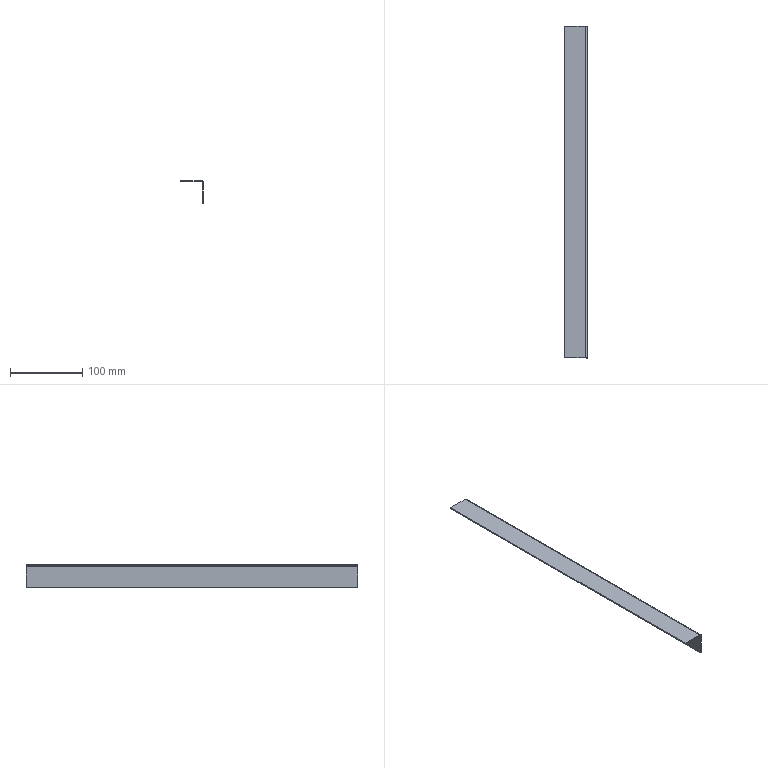Part | SolidWorks | features BaseBody 1 | 1 solid | 10 faces | box 31.5 x 460 x 31.5 mm | volume 41769 mm3 | plane 8 | cylinder 2 | commonest cylinder face diameters 3 x1 6 x1
STEP:
#1=CARTESIAN_POINT('',(0.,460.,-30.));
#2=VERTEX_POINT('',#1);
#3=CARTESIAN_POINT('',(0.,460.,-1.5));
#4=VERTEX_POINT('',#3);
#5=CARTESIAN_POINT('',(0.,460.,0.1965));
#6=DIRECTION('',(0.,0.,1.));
#7=VECTOR('',#6,1000.);
#8=LINE('',#5,#7);
#9=EDGE_CURVE('',#2,#4,#8,.T.);
#10=ORIENTED_EDGE('',*,*,#9,.F.);
#11=CARTESIAN_POINT('',(0.,0.,-30.));
#12=VERTEX_POINT('',#11);
#13=CARTESIAN_POINT('',(0.,230.,-30.));
#14=DIRECTION('',(0.,1.,0.));
#15=VECTOR('',#14,1000.);
#16=LINE('',#13,#15);
#17=EDGE_CURVE('',#12,#2,#16,.T.);
#18=ORIENTED_EDGE('',*,*,#17,.F.);
#19=CARTESIAN_POINT('',(0.,0.,-1.5));
#20=VERTEX_POINT('',#19);
#21=CARTESIAN_POINT('',(0.,0.,0.1965));
#22=DIRECTION('',(0.,0.,-1.));
#23=VECTOR('',#22,1000.);
#24=LINE('',#21,#23);
#25=EDGE_CURVE('',#20,#12,#24,.T.);
#26=ORIENTED_EDGE('',*,*,#25,.F.);
#27=CARTESIAN_POINT('',(0.,230.,-1.5));
#28=DIRECTION('',(0.,-1.,0.));
#29=VECTOR('',#28,1000.);
#30=LINE('',#27,#29);
#31=EDGE_CURVE('',#4,#20,#30,.T.);
#32=ORIENTED_EDGE('',*,*,#31,.F.);
#33=EDGE_LOOP('',(#10,#18,#26,#32));
#34=FACE_OUTER_BOUND('',#33,.T.);
#35=CARTESIAN_POINT('',(0.,230.,0.1965));
#36=DIRECTION('',(1.,0.,0.));
#37=DIRECTION('',(0.,0.,-1.));
#38=AXIS2_PLACEMENT_3D('',#35,#36,#37);
#39=PLANE('',#38);
#40=ADVANCED_FACE('',(#34),#39,.F.);
#41=CARTESIAN_POINT('',(-1.5,0.,0.));
#42=VERTEX_POINT('',#41);
#43=CARTESIAN_POINT('',(-1.5,0.,-1.5));
#44=DIRECTION('',(0.,1.,0.));
#45=DIRECTION('',(0.,0.,1.));
#46=AXIS2_PLACEMENT_3D('',#43,#44,#45);
#47=CIRCLE('',#46,1.5);
#48=EDGE_CURVE('',#42,#20,#47,.T.);
#49=ORIENTED_EDGE('',*,*,#48,.F.);
#50=CARTESIAN_POINT('',(-1.5,460.,0.));
#51=VERTEX_POINT('',#50);
#52=CARTESIAN_POINT('',(-1.5,230.,0.));
#53=DIRECTION('',(0.,-1.,0.));
#54=VECTOR('',#53,1000.);
#55=LINE('',#52,#54);
#56=EDGE_CURVE('',#51,#42,#55,.T.);
#57=ORIENTED_EDGE('',*,*,#56,.F.);
#58=CARTESIAN_POINT('',(-1.5,460.,-1.5));
#59=DIRECTION('',(0.,-1.,0.));
#60=DIRECTION('',(0.,0.,1.));
#61=AXIS2_PLACEMENT_3D('',#58,#59,#60);
#62=CIRCLE('',#61,1.5);
#63=EDGE_CURVE('',#4,#51,#62,.T.);
#64=ORIENTED_EDGE('',*,*,#63,.F.);
#65=ORIENTED_EDGE('',*,*,#31,.T.);
#66=EDGE_LOOP('',(#49,#57,#64,#65));
#67=FACE_OUTER_BOUND('',#66,.T.);
#68=CARTESIAN_POINT('',(-1.5,230.,-1.5));
#69=DIRECTION('',(0.,1.,0.));
#70=DIRECTION('',(0.,0.,1.));
#71=AXIS2_PLACEMENT_3D('',#68,#69,#70);
#72=CYLINDRICAL_SURFACE('',#71,1.5);
#73=ADVANCED_FACE('',(#67),#72,.F.);
#74=CARTESIAN_POINT('',(1.5,460.,-30.));
#75=VERTEX_POINT('',#74);
#76=CARTESIAN_POINT('',(1.5,460.,-30.));
#77=DIRECTION('',(-1.,0.,0.));
#78=VECTOR('',#77,1000.);
#79=LINE('',#76,#78);
#80=EDGE_CURVE('',#75,#2,#79,.T.);
#81=ORIENTED_EDGE('',*,*,#80,.T.);
#82=ORIENTED_EDGE('',*,*,#9,.T.);
#83=ORIENTED_EDGE('',*,*,#63,.T.);
#84=CARTESIAN_POINT('',(-30.,460.,0.));
#85=VERTEX_POINT('',#84);
#86=CARTESIAN_POINT('',(0.1965,460.,0.));
#87=DIRECTION('',(-1.,0.,0.));
#88=VECTOR('',#87,1000.);
#89=LINE('',#86,#88);
#90=EDGE_CURVE('',#51,#85,#89,.T.);
#91=ORIENTED_EDGE('',*,*,#90,.T.);
#92=CARTESIAN_POINT('',(-30.,460.,1.5));
#93=VERTEX_POINT('',#92);
#94=CARTESIAN_POINT('',(-30.,460.,1.5));
#95=DIRECTION('',(0.,0.,-1.));
#96=VECTOR('',#95,1000.);
#97=LINE('',#94,#96);
#98=EDGE_CURVE('',#93,#85,#97,.T.);
#99=ORIENTED_EDGE('',*,*,#98,.F.);
#100=CARTESIAN_POINT('',(-1.5,460.,1.5));
#101=VERTEX_POINT('',#100);
#102=CARTESIAN_POINT('',(-1.5,460.,1.5));
#103=DIRECTION('',(1.,0.,0.));
#104=VECTOR('',#103,1000.);
#105=LINE('',#102,#104);
#106=EDGE_CURVE('',#93,#101,#105,.T.);
#107=ORIENTED_EDGE('',*,*,#106,.T.);
#108=CARTESIAN_POINT('',(1.5,460.,-1.5));
#109=VERTEX_POINT('',#108);
#110=CARTESIAN_POINT('',(-1.5,460.,-1.5));
#111=DIRECTION('',(0.,1.,0.));
#112=DIRECTION('',(0.,0.,1.));
#113=AXIS2_PLACEMENT_3D('',#110,#111,#112);
#114=CIRCLE('',#113,3.);
#115=EDGE_CURVE('',#101,#109,#114,.T.);
#116=ORIENTED_EDGE('',*,*,#115,.T.);
#117=CARTESIAN_POINT('',(1.5,460.,1.893));
#118=DIRECTION('',(0.,0.,-1.));
#119=VECTOR('',#118,1000.);
#120=LINE('',#117,#119);
#121=EDGE_CURVE('',#109,#75,#120,.T.);
#122=ORIENTED_EDGE('',*,*,#121,.T.);
#123=EDGE_LOOP('',(#81,#82,#83,#91,#99,#107,#116,#122));
#124=FACE_OUTER_BOUND('',#123,.T.);
#125=CARTESIAN_POINT('',(1.5,460.,1.893));
#126=DIRECTION('',(0.,1.,0.));
#127=DIRECTION('',(0.,0.,1.));
#128=AXIS2_PLACEMENT_3D('',#125,#126,#127);
#129=PLANE('',#128);
#130=ADVANCED_FACE('',(#124),#129,.T.);
#131=CARTESIAN_POINT('',(1.5,0.,-30.));
#132=VERTEX_POINT('',#131);
#133=CARTESIAN_POINT('',(1.5,0.,-30.));
#134=DIRECTION('',(0.,-1.,0.));
#135=VECTOR('',#134,1000.);
#136=LINE('',#133,#135);
#137=EDGE_CURVE('',#75,#132,#136,.T.);
#138=ORIENTED_EDGE('',*,*,#137,.T.);
#139=CARTESIAN_POINT('',(1.5,0.,-30.));
#140=DIRECTION('',(-1.,0.,0.));
#141=VECTOR('',#140,1000.);
#142=LINE('',#139,#141);
#143=EDGE_CURVE('',#132,#12,#142,.T.);
#144=ORIENTED_EDGE('',*,*,#143,.T.);
#145=ORIENTED_EDGE('',*,*,#17,.T.);
#146=ORIENTED_EDGE('',*,*,#80,.F.);
#147=EDGE_LOOP('',(#138,#144,#145,#146));
#148=FACE_OUTER_BOUND('',#147,.T.);
#149=CARTESIAN_POINT('',(1.5,0.,-30.));
#150=DIRECTION('',(0.,0.,-1.));
#151=DIRECTION('',(-1.,0.,0.));
#152=AXIS2_PLACEMENT_3D('',#149,#150,#151);
#153=PLANE('',#152);
#154=ADVANCED_FACE('',(#148),#153,.T.);
#155=ORIENTED_EDGE('',*,*,#143,.F.);
#156=CARTESIAN_POINT('',(1.5,0.,-1.5));
#157=VERTEX_POINT('',#156);
#158=CARTESIAN_POINT('',(1.5,0.,-1.5));
#159=DIRECTION('',(0.,0.,1.));
#160=VECTOR('',#159,1000.);
#161=LINE('',#158,#160);
#162=EDGE_CURVE('',#132,#157,#161,.T.);
#163=ORIENTED_EDGE('',*,*,#162,.T.);
#164=CARTESIAN_POINT('',(-1.5,0.,1.5));
#165=VERTEX_POINT('',#164);
#166=CARTESIAN_POINT('',(-1.5,0.,-1.5));
#167=DIRECTION('',(0.,-1.,0.));
#168=DIRECTION('',(0.,0.,1.));
#169=AXIS2_PLACEMENT_3D('',#166,#167,#168);
#170=CIRCLE('',#169,3.);
#171=EDGE_CURVE('',#157,#165,#170,.T.);
#172=ORIENTED_EDGE('',*,*,#171,.T.);
#173=CARTESIAN_POINT('',(-30.,0.,1.5));
#174=VERTEX_POINT('',#173);
#175=CARTESIAN_POINT('',(1.893,0.,1.5));
#176=DIRECTION('',(-1.,0.,0.));
#177=VECTOR('',#176,1000.);
#178=LINE('',#175,#177);
#179=EDGE_CURVE('',#165,#174,#178,.T.);
#180=ORIENTED_EDGE('',*,*,#179,.T.);
#181=CARTESIAN_POINT('',(-30.,0.,0.));
#182=VERTEX_POINT('',#181);
#183=CARTESIAN_POINT('',(-30.,0.,1.5));
#184=DIRECTION('',(0.,0.,-1.));
#185=VECTOR('',#184,1000.);
#186=LINE('',#183,#185);
#187=EDGE_CURVE('',#174,#182,#186,.T.);
#188=ORIENTED_EDGE('',*,*,#187,.T.);
#189=CARTESIAN_POINT('',(0.1965,0.,0.));
#190=DIRECTION('',(1.,0.,0.));
#191=VECTOR('',#190,1000.);
#192=LINE('',#189,#191);
#193=EDGE_CURVE('',#182,#42,#192,.T.);
#194=ORIENTED_EDGE('',*,*,#193,.T.);
#195=ORIENTED_EDGE('',*,*,#48,.T.);
#196=ORIENTED_EDGE('',*,*,#25,.T.);
#197=EDGE_LOOP('',(#155,#163,#172,#180,#188,#194,#195,#196));
#198=FACE_OUTER_BOUND('',#197,.T.);
#199=CARTESIAN_POINT('',(1.5,0.,-1.5));
#200=DIRECTION('',(0.,-1.,0.));
#201=DIRECTION('',(0.,0.,-1.));
#202=AXIS2_PLACEMENT_3D('',#199,#200,#201);
#203=PLANE('',#202);
#204=ADVANCED_FACE('',(#198),#203,.T.);
#205=ORIENTED_EDGE('',*,*,#193,.F.);
#206=CARTESIAN_POINT('',(-30.,230.,0.));
#207=DIRECTION('',(0.,-1.,0.));
#208=VECTOR('',#207,1000.);
#209=LINE('',#206,#208);
#210=EDGE_CURVE('',#85,#182,#209,.T.);
#211=ORIENTED_EDGE('',*,*,#210,.F.);
#212=ORIENTED_EDGE('',*,*,#90,.F.);
#213=ORIENTED_EDGE('',*,*,#56,.T.);
#214=EDGE_LOOP('',(#205,#211,#212,#213));
#215=FACE_OUTER_BOUND('',#214,.T.);
#216=CARTESIAN_POINT('',(0.1965,230.,0.));
#217=DIRECTION('',(0.,0.,1.));
#218=DIRECTION('',(1.,0.,0.));
#219=AXIS2_PLACEMENT_3D('',#216,#217,#218);
#220=PLANE('',#219);
#221=ADVANCED_FACE('',(#215),#220,.F.);
#222=ORIENTED_EDGE('',*,*,#137,.F.);
#223=ORIENTED_EDGE('',*,*,#121,.F.);
#224=CARTESIAN_POINT('',(1.5,230.,-1.5));
#225=DIRECTION('',(0.,-1.,0.));
#226=VECTOR('',#225,1000.);
#227=LINE('',#224,#226);
#228=EDGE_CURVE('',#109,#157,#227,.T.);
#229=ORIENTED_EDGE('',*,*,#228,.T.);
#230=ORIENTED_EDGE('',*,*,#162,.F.);
#231=EDGE_LOOP('',(#222,#223,#229,#230));
#232=FACE_OUTER_BOUND('',#231,.T.);
#233=CARTESIAN_POINT('',(1.5,230.,0.1965));
#234=DIRECTION('',(1.,0.,0.));
#235=DIRECTION('',(0.,0.,-1.));
#236=AXIS2_PLACEMENT_3D('',#233,#234,#235);
#237=PLANE('',#236);
#238=ADVANCED_FACE('',(#232),#237,.T.);
#239=CARTESIAN_POINT('',(-1.5,230.,1.5));
#240=DIRECTION('',(0.,-1.,0.));
#241=VECTOR('',#240,1000.);
#242=LINE('',#239,#241);
#243=EDGE_CURVE('',#101,#165,#242,.T.);
#244=ORIENTED_EDGE('',*,*,#243,.T.);
#245=ORIENTED_EDGE('',*,*,#171,.F.);
#246=ORIENTED_EDGE('',*,*,#228,.F.);
#247=ORIENTED_EDGE('',*,*,#115,.F.);
#248=EDGE_LOOP('',(#244,#245,#246,#247));
#249=FACE_OUTER_BOUND('',#248,.T.);
#250=CARTESIAN_POINT('',(-1.5,230.,-1.5));
#251=DIRECTION('',(0.,1.,0.));
#252=DIRECTION('',(0.,0.,1.));
#253=AXIS2_PLACEMENT_3D('',#250,#251,#252);
#254=CYLINDRICAL_SURFACE('',#253,3.);
#255=ADVANCED_FACE('',(#249),#254,.T.);
#256=CARTESIAN_POINT('',(-30.,460.,1.5));
#257=DIRECTION('',(0.,1.,0.));
#258=VECTOR('',#257,1000.);
#259=LINE('',#256,#258);
#260=EDGE_CURVE('',#174,#93,#259,.T.);
#261=ORIENTED_EDGE('',*,*,#260,.T.);
#262=ORIENTED_EDGE('',*,*,#98,.T.);
#263=ORIENTED_EDGE('',*,*,#210,.T.);
#264=ORIENTED_EDGE('',*,*,#187,.F.);
#265=EDGE_LOOP('',(#261,#262,#263,#264));
#266=FACE_OUTER_BOUND('',#265,.T.);
#267=CARTESIAN_POINT('',(-30.,460.,1.5));
#268=DIRECTION('',(-1.,0.,0.));
#269=DIRECTION('',(0.,0.,1.));
#270=AXIS2_PLACEMENT_3D('',#267,#268,#269);
#271=PLANE('',#270);
#272=ADVANCED_FACE('',(#266),#271,.T.);
#273=ORIENTED_EDGE('',*,*,#260,.F.);
#274=ORIENTED_EDGE('',*,*,#179,.F.);
#275=ORIENTED_EDGE('',*,*,#243,.F.);
#276=ORIENTED_EDGE('',*,*,#106,.F.);
#277=EDGE_LOOP('',(#273,#274,#275,#276));
#278=FACE_OUTER_BOUND('',#277,.T.);
#279=CARTESIAN_POINT('',(0.1965,230.,1.5));
#280=DIRECTION('',(0.,0.,1.));
#281=DIRECTION('',(1.,0.,0.));
#282=AXIS2_PLACEMENT_3D('',#279,#280,#281);
#283=PLANE('',#282);
#284=ADVANCED_FACE('',(#278),#283,.T.);
#285=CLOSED_SHELL('',(#40,#73,#130,#154,#204,#221,#238,#255,#272,#284));
#286=MANIFOLD_SOLID_BREP('',#285);
#287=CARTESIAN_POINT('',(0.,0.,0.));
#288=DIRECTION('',(0.,0.,1.));
#289=DIRECTION('',(1.,0.,0.));
#290=AXIS2_PLACEMENT_3D('',#287,#288,#289);
#291=(LENGTH_UNIT()NAMED_UNIT(*)SI_UNIT(.MILLI.,.METRE.));
#292=UNCERTAINTY_MEASURE_WITH_UNIT(LENGTH_MEASURE(0.00001),#291,'','');
#293=(NAMED_UNIT(*)PLANE_ANGLE_UNIT()SI_UNIT($,.RADIAN.));
#294=(NAMED_UNIT(*)SI_UNIT($,.STERADIAN.)SOLID_ANGLE_UNIT());
#295=(GEOMETRIC_REPRESENTATION_CONTEXT(3)GLOBAL_UNCERTAINTY_ASSIGNED_CONTEXT((#292))GLOBAL_UNIT_ASSIGNED_CONTEXT((#291,#293,#294))REPRESENTATION_CONTEXT('',''));
#296=ADVANCED_BREP_SHAPE_REPRESENTATION('',(#286,#290),#295);